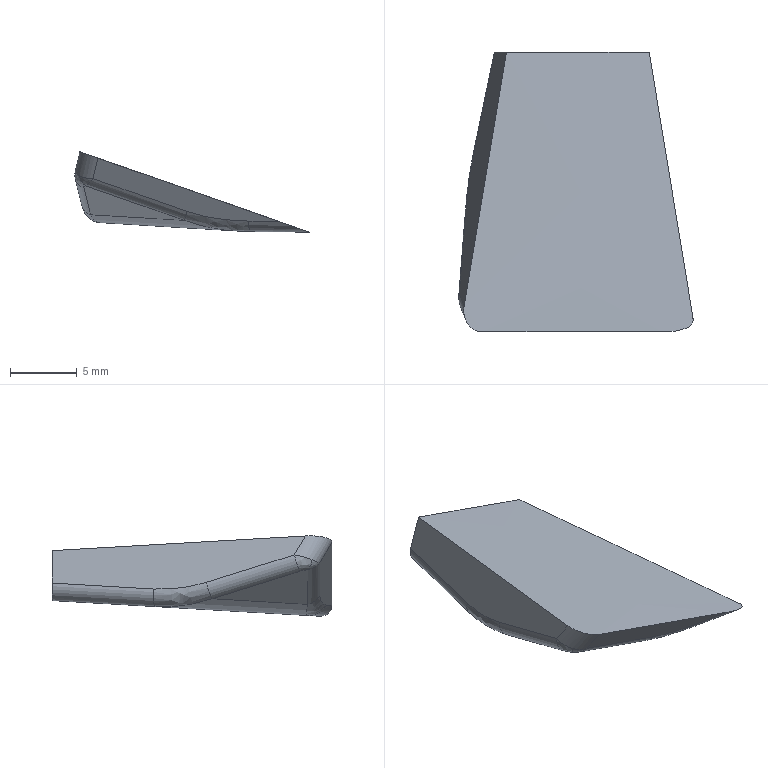Part | STEP file | solid 26 | 1 solid | 16 faces | box 17.629 x 21.043 x 6.038 mm | volume 691.957 mm3 | cylinder 6 | plane 5 | spline 4 | other 1 | commonest cylinder face diameters 3 x3 2 x2 16 x1